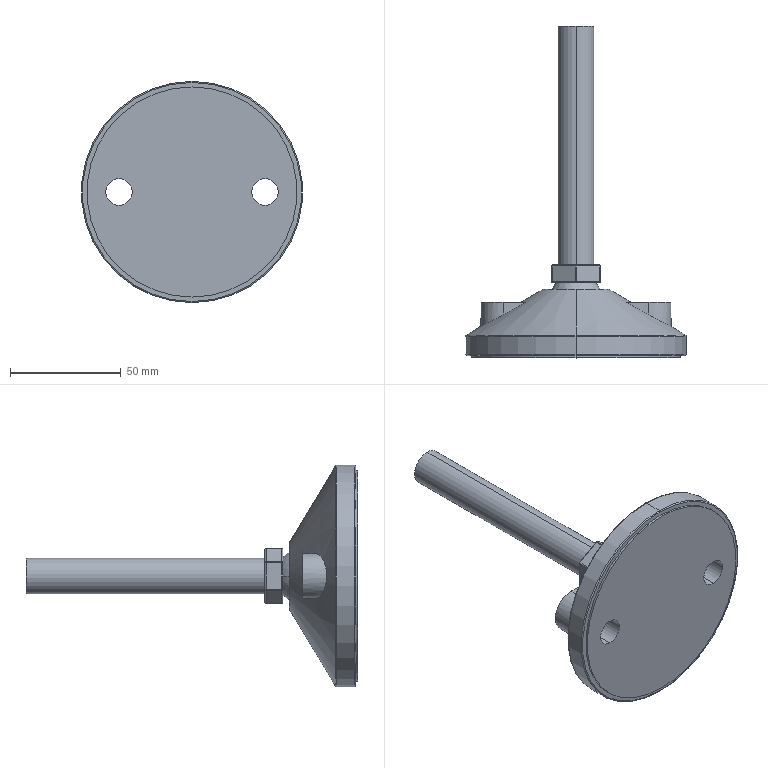Part | STEP file | BASE_Foot_GFTR16-100-100 | 1 solid | 69 faces | box 100 x 150 x 100 mm | volume 177771 mm3 | cylinder 31 | plane 18 | sphere 14 | torus 4 | cone 2 | commonest cylinder face diameters 1 x19 12 x4 16 x2 20 x2 95 x2 100 x2